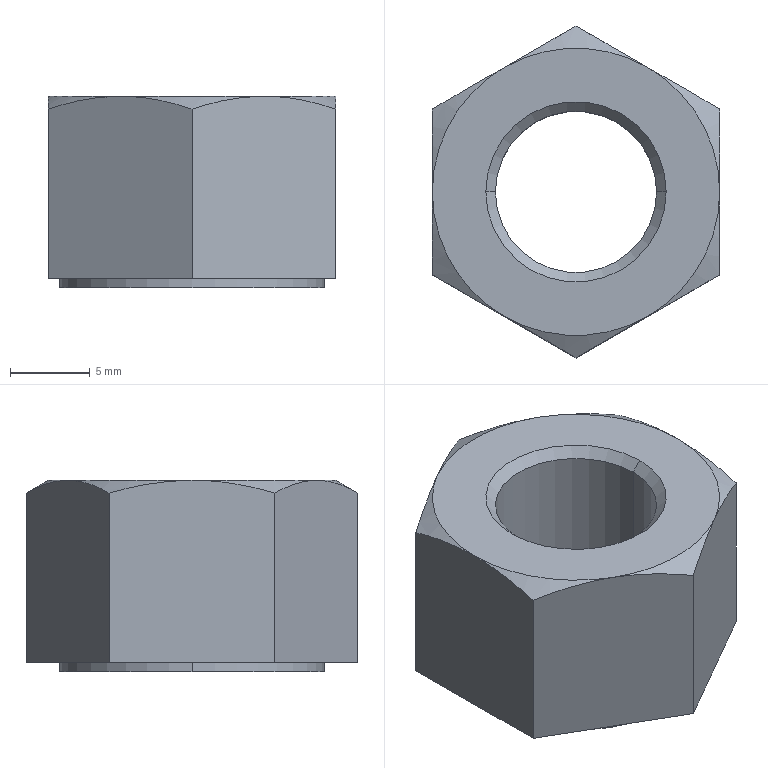Part | SolidWorks | 1 solid | 23 faces | box 18 x 20.785 x 12 mm | volume 2348 mm3 | cone 10 | plane 9 | cylinder 4 | commonest cylinder face diameters 10.106 x2 16.6 x2
STEP:
#1=CARTESIAN_POINT('',(-5.053,0.,11.4));
#2=VERTEX_POINT('',#1);
#3=CARTESIAN_POINT('',(5.053,0.,11.4));
#4=VERTEX_POINT('',#3);
#5=CARTESIAN_POINT('',(0.,0.,11.4));
#6=DIRECTION('',(0.,0.,1.));
#7=DIRECTION('',(-1.,0.,0.));
#8=AXIS2_PLACEMENT_3D('',#5,#6,#7);
#9=CIRCLE('',#8,5.053);
#10=EDGE_CURVE('',#2,#4,#9,.T.);
#11=ORIENTED_EDGE('',*,*,#10,.F.);
#12=CARTESIAN_POINT('',(-5.653,0.,12.));
#13=VERTEX_POINT('',#12);
#14=CARTESIAN_POINT('',(-5.053,0.,11.4));
#15=DIRECTION('',(-0.7071,0.,0.7071));
#16=VECTOR('',#15,1000.);
#17=LINE('',#14,#16);
#18=EDGE_CURVE('',#2,#13,#17,.T.);
#19=ORIENTED_EDGE('',*,*,#18,.T.);
#20=CARTESIAN_POINT('',(5.653,0.,12.));
#21=VERTEX_POINT('',#20);
#22=CARTESIAN_POINT('',(0.,0.,12.));
#23=DIRECTION('',(0.,0.,-1.));
#24=DIRECTION('',(-1.,0.,0.));
#25=AXIS2_PLACEMENT_3D('',#22,#23,#24);
#26=CIRCLE('',#25,5.653);
#27=EDGE_CURVE('',#21,#13,#26,.T.);
#28=ORIENTED_EDGE('',*,*,#27,.F.);
#29=CARTESIAN_POINT('',(5.053,0.,11.4));
#30=DIRECTION('',(0.7071,0.,0.7071));
#31=VECTOR('',#30,1000.);
#32=LINE('',#29,#31);
#33=EDGE_CURVE('',#4,#21,#32,.T.);
#34=ORIENTED_EDGE('',*,*,#33,.F.);
#35=EDGE_LOOP('',(#11,#19,#28,#34));
#36=FACE_OUTER_BOUND('',#35,.T.);
#37=CARTESIAN_POINT('',(0.,0.,11.4));
#38=DIRECTION('',(0.,0.,1.));
#39=DIRECTION('',(1.,0.,0.));
#40=AXIS2_PLACEMENT_3D('',#37,#38,#39);
#41=CONICAL_SURFACE('',#40,5.053,0.7854);
#42=ADVANCED_FACE('',(#36),#41,.F.);
#43=CARTESIAN_POINT('',(5.053,0.,0.6));
#44=VERTEX_POINT('',#43);
#45=CARTESIAN_POINT('',(-5.053,0.,0.6));
#46=VERTEX_POINT('',#45);
#47=CARTESIAN_POINT('',(0.,0.,0.6));
#48=DIRECTION('',(0.,0.,-1.));
#49=DIRECTION('',(-1.,0.,0.));
#50=AXIS2_PLACEMENT_3D('',#47,#48,#49);
#51=CIRCLE('',#50,5.053);
#52=EDGE_CURVE('',#44,#46,#51,.T.);
#53=ORIENTED_EDGE('',*,*,#52,.F.);
#54=CARTESIAN_POINT('',(5.653,0.,0.));
#55=VERTEX_POINT('',#54);
#56=CARTESIAN_POINT('',(5.653,0.,0.));
#57=DIRECTION('',(0.7071,0.,-0.7071));
#58=VECTOR('',#57,1000.);
#59=LINE('',#56,#58);
#60=EDGE_CURVE('',#44,#55,#59,.T.);
#61=ORIENTED_EDGE('',*,*,#60,.T.);
#62=CARTESIAN_POINT('',(-5.653,0.,0.));
#63=VERTEX_POINT('',#62);
#64=CARTESIAN_POINT('',(0.,0.,0.));
#65=DIRECTION('',(0.,0.,1.));
#66=DIRECTION('',(-1.,0.,0.));
#67=AXIS2_PLACEMENT_3D('',#64,#65,#66);
#68=CIRCLE('',#67,5.653);
#69=EDGE_CURVE('',#63,#55,#68,.T.);
#70=ORIENTED_EDGE('',*,*,#69,.F.);
#71=CARTESIAN_POINT('',(-5.653,0.,0.));
#72=DIRECTION('',(-0.7071,0.,-0.7071));
#73=VECTOR('',#72,1000.);
#74=LINE('',#71,#73);
#75=EDGE_CURVE('',#46,#63,#74,.T.);
#76=ORIENTED_EDGE('',*,*,#75,.F.);
#77=EDGE_LOOP('',(#53,#61,#70,#76));
#78=FACE_OUTER_BOUND('',#77,.T.);
#79=CARTESIAN_POINT('',(0.,0.,0.));
#80=DIRECTION('',(0.,0.,-1.));
#81=DIRECTION('',(-1.,0.,0.));
#82=AXIS2_PLACEMENT_3D('',#79,#80,#81);
#83=CONICAL_SURFACE('',#82,5.653,0.7854);
#84=ADVANCED_FACE('',(#78),#83,.F.);
#85=CARTESIAN_POINT('',(8.3,0.,0.6));
#86=VERTEX_POINT('',#85);
#87=CARTESIAN_POINT('',(-8.3,0.,0.6));
#88=VERTEX_POINT('',#87);
#89=CARTESIAN_POINT('',(0.,0.,0.6));
#90=DIRECTION('',(0.,0.,1.));
#91=DIRECTION('',(1.,0.,0.));
#92=AXIS2_PLACEMENT_3D('',#89,#90,#91);
#93=CIRCLE('',#92,8.3);
#94=EDGE_CURVE('',#86,#88,#93,.T.);
#95=ORIENTED_EDGE('',*,*,#94,.F.);
#96=CARTESIAN_POINT('',(8.3,0.,0.));
#97=VERTEX_POINT('',#96);
#98=CARTESIAN_POINT('',(8.3,0.,0.6));
#99=DIRECTION('',(0.,0.,-1.));
#100=VECTOR('',#99,1000.);
#101=LINE('',#98,#100);
#102=EDGE_CURVE('',#86,#97,#101,.T.);
#103=ORIENTED_EDGE('',*,*,#102,.T.);
#104=CARTESIAN_POINT('',(-8.3,0.,0.));
#105=VERTEX_POINT('',#104);
#106=CARTESIAN_POINT('',(0.,0.,0.));
#107=DIRECTION('',(0.,0.,1.));
#108=DIRECTION('',(1.,0.,0.));
#109=AXIS2_PLACEMENT_3D('',#106,#107,#108);
#110=CIRCLE('',#109,8.3);
#111=EDGE_CURVE('',#97,#105,#110,.T.);
#112=ORIENTED_EDGE('',*,*,#111,.T.);
#113=CARTESIAN_POINT('',(-8.3,0.,0.6));
#114=DIRECTION('',(0.,0.,-1.));
#115=VECTOR('',#114,1000.);
#116=LINE('',#113,#115);
#117=EDGE_CURVE('',#88,#105,#116,.T.);
#118=ORIENTED_EDGE('',*,*,#117,.F.);
#119=EDGE_LOOP('',(#95,#103,#112,#118));
#120=FACE_OUTER_BOUND('',#119,.T.);
#121=CARTESIAN_POINT('',(0.,0.,0.6));
#122=DIRECTION('',(0.,0.,-1.));
#123=DIRECTION('',(-1.,0.,0.));
#124=AXIS2_PLACEMENT_3D('',#121,#122,#123);
#125=CYLINDRICAL_SURFACE('',#124,8.3);
#126=ADVANCED_FACE('',(#120),#125,.T.);
#127=ORIENTED_EDGE('',*,*,#10,.T.);
#128=CARTESIAN_POINT('',(5.053,0.,12.));
#129=DIRECTION('',(0.,0.,-1.));
#130=VECTOR('',#129,1000.);
#131=LINE('',#128,#130);
#132=EDGE_CURVE('',#4,#44,#131,.T.);
#133=ORIENTED_EDGE('',*,*,#132,.T.);
#134=ORIENTED_EDGE('',*,*,#52,.T.);
#135=CARTESIAN_POINT('',(-5.053,0.,12.));
#136=DIRECTION('',(0.,0.,-1.));
#137=VECTOR('',#136,1000.);
#138=LINE('',#135,#137);
#139=EDGE_CURVE('',#2,#46,#138,.T.);
#140=ORIENTED_EDGE('',*,*,#139,.F.);
#141=EDGE_LOOP('',(#127,#133,#134,#140));
#142=FACE_OUTER_BOUND('',#141,.T.);
#143=CARTESIAN_POINT('',(0.,0.,12.));
#144=DIRECTION('',(0.,0.,-1.));
#145=DIRECTION('',(-1.,0.,0.));
#146=AXIS2_PLACEMENT_3D('',#143,#144,#145);
#147=CYLINDRICAL_SURFACE('',#146,5.053);
#148=ADVANCED_FACE('',(#142),#147,.F.);
#149=ORIENTED_EDGE('',*,*,#27,.T.);
#150=CARTESIAN_POINT('',(0.,0.,12.));
#151=DIRECTION('',(0.,0.,-1.));
#152=DIRECTION('',(-1.,0.,0.));
#153=AXIS2_PLACEMENT_3D('',#150,#151,#152);
#154=CIRCLE('',#153,5.653);
#155=EDGE_CURVE('',#13,#21,#154,.T.);
#156=ORIENTED_EDGE('',*,*,#155,.T.);
#157=EDGE_LOOP('',(#149,#156));
#158=FACE_BOUND('',#157,.T.);
#159=CARTESIAN_POINT('',(-4.5,7.794,12.));
#160=VERTEX_POINT('',#159);
#161=CARTESIAN_POINT('',(-9.,0.,12.));
#162=VERTEX_POINT('',#161);
#163=CARTESIAN_POINT('',(0.,0.,12.));
#164=DIRECTION('',(0.,0.,1.));
#165=DIRECTION('',(1.,0.,0.));
#166=AXIS2_PLACEMENT_3D('',#163,#164,#165);
#167=CIRCLE('',#166,9.);
#168=EDGE_CURVE('',#160,#162,#167,.T.);
#169=ORIENTED_EDGE('',*,*,#168,.T.);
#170=CARTESIAN_POINT('',(-4.5,-7.794,12.));
#171=VERTEX_POINT('',#170);
#172=CARTESIAN_POINT('',(0.,0.,12.));
#173=DIRECTION('',(0.,0.,1.));
#174=DIRECTION('',(1.,0.,0.));
#175=AXIS2_PLACEMENT_3D('',#172,#173,#174);
#176=CIRCLE('',#175,9.);
#177=EDGE_CURVE('',#162,#171,#176,.T.);
#178=ORIENTED_EDGE('',*,*,#177,.T.);
#179=CARTESIAN_POINT('',(4.5,-7.794,12.));
#180=VERTEX_POINT('',#179);
#181=CARTESIAN_POINT('',(0.,0.,12.));
#182=DIRECTION('',(0.,0.,1.));
#183=DIRECTION('',(1.,0.,0.));
#184=AXIS2_PLACEMENT_3D('',#181,#182,#183);
#185=CIRCLE('',#184,9.);
#186=EDGE_CURVE('',#171,#180,#185,.T.);
#187=ORIENTED_EDGE('',*,*,#186,.T.);
#188=CARTESIAN_POINT('',(9.,0.,12.));
#189=VERTEX_POINT('',#188);
#190=CARTESIAN_POINT('',(0.,0.,12.));
#191=DIRECTION('',(0.,0.,1.));
#192=DIRECTION('',(1.,0.,0.));
#193=AXIS2_PLACEMENT_3D('',#190,#191,#192);
#194=CIRCLE('',#193,9.);
#195=EDGE_CURVE('',#180,#189,#194,.T.);
#196=ORIENTED_EDGE('',*,*,#195,.T.);
#197=CARTESIAN_POINT('',(4.5,7.794,12.));
#198=VERTEX_POINT('',#197);
#199=CARTESIAN_POINT('',(0.,0.,12.));
#200=DIRECTION('',(0.,0.,1.));
#201=DIRECTION('',(1.,0.,0.));
#202=AXIS2_PLACEMENT_3D('',#199,#200,#201);
#203=CIRCLE('',#202,9.);
#204=EDGE_CURVE('',#189,#198,#203,.T.);
#205=ORIENTED_EDGE('',*,*,#204,.T.);
#206=CARTESIAN_POINT('',(0.,0.,12.));
#207=DIRECTION('',(0.,0.,1.));
#208=DIRECTION('',(1.,0.,0.));
#209=AXIS2_PLACEMENT_3D('',#206,#207,#208);
#210=CIRCLE('',#209,9.);
#211=EDGE_CURVE('',#198,#160,#210,.T.);
#212=ORIENTED_EDGE('',*,*,#211,.T.);
#213=EDGE_LOOP('',(#169,#178,#187,#196,#205,#212));
#214=FACE_OUTER_BOUND('',#213,.T.);
#215=CARTESIAN_POINT('',(9.,5.196,12.));
#216=DIRECTION('',(0.,0.,-1.));
#217=DIRECTION('',(-1.,0.,0.));
#218=AXIS2_PLACEMENT_3D('',#215,#216,#217);
#219=PLANE('',#218);
#220=ADVANCED_FACE('',(#158,#214),#219,.F.);
#221=CARTESIAN_POINT('',(9.,5.196,11.196));
#222=VERTEX_POINT('',#221);
#223=CARTESIAN_POINT('',(9.,5.196,11.196));
#224=CARTESIAN_POINT('',(8.264,5.621,11.442));
#225=CARTESIAN_POINT('',(7.522,6.049,11.644));
#226=CARTESIAN_POINT('',(6.024,6.914,11.923));
#227=CARTESIAN_POINT('',(5.267,7.352,12.));
#228=CARTESIAN_POINT('',(4.5,7.794,12.));
#229=B_SPLINE_CURVE_WITH_KNOTS('',3,(#223,#224,#225,#226,#227,#228),.UNSPECIFIED.,.F.,.F.,(4,2,4),(0.000000238,0.002629,0.005258),.UNSPECIFIED.);
#230=EDGE_CURVE('',#222,#198,#229,.T.);
#231=ORIENTED_EDGE('',*,*,#230,.F.);
#232=CARTESIAN_POINT('',(9.,5.196,0.6));
#233=VERTEX_POINT('',#232);
#234=CARTESIAN_POINT('',(9.,5.196,12.));
#235=DIRECTION('',(0.,0.,-1.));
#236=VECTOR('',#235,1000.);
#237=LINE('',#234,#236);
#238=EDGE_CURVE('',#222,#233,#237,.T.);
#239=ORIENTED_EDGE('',*,*,#238,.T.);
#240=CARTESIAN_POINT('',(0.,10.392,0.6));
#241=VERTEX_POINT('',#240);
#242=CARTESIAN_POINT('',(9.,5.196,0.6));
#243=DIRECTION('',(-0.866,0.5,0.));
#244=VECTOR('',#243,1000.);
#245=LINE('',#242,#244);
#246=EDGE_CURVE('',#233,#241,#245,.T.);
#247=ORIENTED_EDGE('',*,*,#246,.T.);
#248=CARTESIAN_POINT('',(0.,10.392,11.196));
#249=VERTEX_POINT('',#248);
#250=CARTESIAN_POINT('',(0.,10.392,12.));
#251=DIRECTION('',(0.,0.,-1.));
#252=VECTOR('',#251,1000.);
#253=LINE('',#250,#252);
#254=EDGE_CURVE('',#249,#241,#253,.T.);
#255=ORIENTED_EDGE('',*,*,#254,.F.);
#256=CARTESIAN_POINT('',(4.5,7.794,12.));
#257=CARTESIAN_POINT('',(4.118,8.015,12.));
#258=CARTESIAN_POINT('',(3.734,8.236,11.981));
#259=CARTESIAN_POINT('',(2.976,8.674,11.907));
#260=CARTESIAN_POINT('',(2.599,8.892,11.853));
#261=CARTESIAN_POINT('',(1.475,9.541,11.643));
#262=CARTESIAN_POINT('',(0.7343,9.968,11.441));
#263=CARTESIAN_POINT('',(0.,10.392,11.196));
#264=B_SPLINE_CURVE_WITH_KNOTS('',3,(#256,#257,#258,#259,#260,#261,#262,#263),.UNSPECIFIED.,.F.,.F.,(4,2,2,4),(0.005258,0.006567,0.007877,0.0105),.UNSPECIFIED.);
#265=EDGE_CURVE('',#198,#249,#264,.T.);
#266=ORIENTED_EDGE('',*,*,#265,.F.);
#267=EDGE_LOOP('',(#231,#239,#247,#255,#266));
#268=FACE_OUTER_BOUND('',#267,.T.);
#269=CARTESIAN_POINT('',(9.,5.196,12.));
#270=DIRECTION('',(-0.5,-0.866,0.));
#271=DIRECTION('',(0.866,-0.5,0.));
#272=AXIS2_PLACEMENT_3D('',#269,#270,#271);
#273=PLANE('',#272);
#274=ADVANCED_FACE('',(#268),#273,.F.);
#275=CARTESIAN_POINT('',(0.,10.392,11.196));
#276=CARTESIAN_POINT('',(-0.7361,9.967,11.442));
#277=CARTESIAN_POINT('',(-1.478,9.539,11.644));
#278=CARTESIAN_POINT('',(-2.976,8.674,11.923));
#279=CARTESIAN_POINT('',(-3.733,8.237,12.));
#280=CARTESIAN_POINT('',(-4.5,7.794,12.));
#281=B_SPLINE_CURVE_WITH_KNOTS('',3,(#275,#276,#277,#278,#279,#280),.UNSPECIFIED.,.F.,.F.,(4,2,4),(0.000000238,0.002629,0.005258),.UNSPECIFIED.);
#282=EDGE_CURVE('',#249,#160,#281,.T.);
#283=ORIENTED_EDGE('',*,*,#282,.F.);
#284=ORIENTED_EDGE('',*,*,#254,.T.);
#285=CARTESIAN_POINT('',(-9.,5.196,0.6));
#286=VERTEX_POINT('',#285);
#287=CARTESIAN_POINT('',(0.,10.392,0.6));
#288=DIRECTION('',(-0.866,-0.5,0.));
#289=VECTOR('',#288,1000.);
#290=LINE('',#287,#289);
#291=EDGE_CURVE('',#241,#286,#290,.T.);
#292=ORIENTED_EDGE('',*,*,#291,.T.);
#293=CARTESIAN_POINT('',(-9.,5.196,11.196));
#294=VERTEX_POINT('',#293);
#295=CARTESIAN_POINT('',(-9.,5.196,12.));
#296=DIRECTION('',(0.,0.,-1.));
#297=VECTOR('',#296,1000.);
#298=LINE('',#295,#297);
#299=EDGE_CURVE('',#294,#286,#298,.T.);
#300=ORIENTED_EDGE('',*,*,#299,.F.);
#301=CARTESIAN_POINT('',(-4.5,7.794,12.));
#302=CARTESIAN_POINT('',(-4.882,7.574,12.));
#303=CARTESIAN_POINT('',(-5.266,7.352,11.981));
#304=CARTESIAN_POINT('',(-6.024,6.914,11.907));
#305=CARTESIAN_POINT('',(-6.401,6.697,11.853));
#306=CARTESIAN_POINT('',(-7.525,6.048,11.643));
#307=CARTESIAN_POINT('',(-8.266,5.62,11.441));
#308=CARTESIAN_POINT('',(-9.,5.196,11.196));
#309=B_SPLINE_CURVE_WITH_KNOTS('',3,(#301,#302,#303,#304,#305,#306,#307,#308),.UNSPECIFIED.,.F.,.F.,(4,2,2,4),(0.005258,0.006567,0.007877,0.0105),.UNSPECIFIED.);
#310=EDGE_CURVE('',#160,#294,#309,.T.);
#311=ORIENTED_EDGE('',*,*,#310,.F.);
#312=EDGE_LOOP('',(#283,#284,#292,#300,#311));
#313=FACE_OUTER_BOUND('',#312,.T.);
#314=CARTESIAN_POINT('',(0.,10.392,12.));
#315=DIRECTION('',(0.5,-0.866,0.));
#316=DIRECTION('',(0.866,0.5,0.));
#317=AXIS2_PLACEMENT_3D('',#314,#315,#316);
#318=PLANE('',#317);
#319=ADVANCED_FACE('',(#313),#318,.F.);
#320=CARTESIAN_POINT('',(-9.,5.196,11.196));
#321=CARTESIAN_POINT('',(-9.,4.356,11.439));
#322=CARTESIAN_POINT('',(-9.,3.505,11.641));
#323=CARTESIAN_POINT('',(-9.,2.204,11.852));
#324=CARTESIAN_POINT('',(-9.,1.766,11.907));
#325=CARTESIAN_POINT('',(-9.,0.8817,11.981));
#326=CARTESIAN_POINT('',(-9.,0.4398,12.));
#327=CARTESIAN_POINT('',(-9.,0.,12.));
#328=B_SPLINE_CURVE_WITH_KNOTS('',3,(#320,#321,#322,#323,#324,#325,#326,#327),.UNSPECIFIED.,.F.,.F.,(4,2,2,4),(0.03023,0.03286,0.03418,0.03549),.UNSPECIFIED.);
#329=EDGE_CURVE('',#294,#162,#328,.T.);
#330=ORIENTED_EDGE('',*,*,#329,.F.);
#331=ORIENTED_EDGE('',*,*,#299,.T.);
#332=CARTESIAN_POINT('',(-9.,-5.196,0.6));
#333=VERTEX_POINT('',#332);
#334=CARTESIAN_POINT('',(-9.,5.196,0.6));
#335=DIRECTION('',(0.,-1.,0.));
#336=VECTOR('',#335,1000.);
#337=LINE('',#334,#336);
#338=EDGE_CURVE('',#286,#333,#337,.T.);
#339=ORIENTED_EDGE('',*,*,#338,.T.);
#340=CARTESIAN_POINT('',(-9.,-5.196,11.196));
#341=VERTEX_POINT('',#340);
#342=CARTESIAN_POINT('',(-9.,-5.196,12.));
#343=DIRECTION('',(0.,0.,-1.));
#344=VECTOR('',#343,1000.);
#345=LINE('',#342,#344);
#346=EDGE_CURVE('',#341,#333,#345,.T.);
#347=ORIENTED_EDGE('',*,*,#346,.F.);
#348=CARTESIAN_POINT('',(-9.,0.,12.));
#349=CARTESIAN_POINT('',(-9.,-0.8789,12.));
#350=CARTESIAN_POINT('',(-9.,-1.751,11.924));
#351=CARTESIAN_POINT('',(-9.,-3.485,11.645));
#352=CARTESIAN_POINT('',(-9.,-4.35,11.44));
#353=CARTESIAN_POINT('',(-9.,-5.196,11.196));
#354=B_SPLINE_CURVE_WITH_KNOTS('',3,(#348,#349,#350,#351,#352,#353),.UNSPECIFIED.,.F.,.F.,(4,2,4),(0.03549,0.03812,0.04075),.UNSPECIFIED.);
#355=EDGE_CURVE('',#162,#341,#354,.T.);
#356=ORIENTED_EDGE('',*,*,#355,.F.);
#357=EDGE_LOOP('',(#330,#331,#339,#347,#356));
#358=FACE_OUTER_BOUND('',#357,.T.);
#359=CARTESIAN_POINT('',(-9.,5.196,12.));
#360=DIRECTION('',(1.,0.,0.));
#361=DIRECTION('',(0.,0.,-1.));
#362=AXIS2_PLACEMENT_3D('',#359,#360,#361);
#363=PLANE('',#362);
#364=ADVANCED_FACE('',(#358),#363,.F.);
#365=CARTESIAN_POINT('',(-9.,-5.196,11.196));
#366=CARTESIAN_POINT('',(-8.264,-5.621,11.442));
#367=CARTESIAN_POINT('',(-7.522,-6.049,11.644));
#368=CARTESIAN_POINT('',(-6.024,-6.914,11.923));
#369=CARTESIAN_POINT('',(-5.267,-7.352,12.));
#370=CARTESIAN_POINT('',(-4.5,-7.794,12.));
#371=B_SPLINE_CURVE_WITH_KNOTS('',3,(#365,#366,#367,#368,#369,#370),.UNSPECIFIED.,.F.,.F.,(4,2,4),(0.000000238,0.002629,0.005258),.UNSPECIFIED.);
#372=EDGE_CURVE('',#341,#171,#371,.T.);
#373=ORIENTED_EDGE('',*,*,#372,.F.);
#374=ORIENTED_EDGE('',*,*,#346,.T.);
#375=CARTESIAN_POINT('',(0.,-10.392,0.6));
#376=VERTEX_POINT('',#375);
#377=CARTESIAN_POINT('',(-9.,-5.196,0.6));
#378=DIRECTION('',(0.866,-0.5,0.));
#379=VECTOR('',#378,1000.);
#380=LINE('',#377,#379);
#381=EDGE_CURVE('',#333,#376,#380,.T.);
#382=ORIENTED_EDGE('',*,*,#381,.T.);
#383=CARTESIAN_POINT('',(0.,-10.392,11.196));
#384=VERTEX_POINT('',#383);
#385=CARTESIAN_POINT('',(0.,-10.392,12.));
#386=DIRECTION('',(0.,0.,-1.));
#387=VECTOR('',#386,1000.);
#388=LINE('',#385,#387);
#389=EDGE_CURVE('',#384,#376,#388,.T.);
#390=ORIENTED_EDGE('',*,*,#389,.F.);
#391=CARTESIAN_POINT('',(-4.5,-7.794,12.));
#392=CARTESIAN_POINT('',(-4.118,-8.015,12.));
#393=CARTESIAN_POINT('',(-3.734,-8.236,11.981));
#394=CARTESIAN_POINT('',(-2.976,-8.674,11.907));
#395=CARTESIAN_POINT('',(-2.599,-8.892,11.853));
#396=CARTESIAN_POINT('',(-1.475,-9.541,11.643));
#397=CARTESIAN_POINT('',(-0.7343,-9.968,11.441));
#398=CARTESIAN_POINT('',(0.,-10.392,11.196));
#399=B_SPLINE_CURVE_WITH_KNOTS('',3,(#391,#392,#393,#394,#395,#396,#397,#398),.UNSPECIFIED.,.F.,.F.,(4,2,2,4),(0.005258,0.006567,0.007877,0.0105),.UNSPECIFIED.);
#400=EDGE_CURVE('',#171,#384,#399,.T.);
#401=ORIENTED_EDGE('',*,*,#400,.F.);
#402=EDGE_LOOP('',(#373,#374,#382,#390,#401));
#403=FACE_OUTER_BOUND('',#402,.T.);
#404=CARTESIAN_POINT('',(-9.,-5.196,12.));
#405=DIRECTION('',(0.5,0.866,0.));
#406=DIRECTION('',(-0.866,0.5,0.));
#407=AXIS2_PLACEMENT_3D('',#404,#405,#406);
#408=PLANE('',#407);
#409=ADVANCED_FACE('',(#403),#408,.F.);
#410=CARTESIAN_POINT('',(0.,-10.392,11.196));
#411=CARTESIAN_POINT('',(0.7361,-9.967,11.442));
#412=CARTESIAN_POINT('',(1.478,-9.539,11.644));
#413=CARTESIAN_POINT('',(2.976,-8.674,11.923));
#414=CARTESIAN_POINT('',(3.733,-8.237,12.));
#415=CARTESIAN_POINT('',(4.5,-7.794,12.));
#416=B_SPLINE_CURVE_WITH_KNOTS('',3,(#410,#411,#412,#413,#414,#415),.UNSPECIFIED.,.F.,.F.,(4,2,4),(0.000000238,0.002629,0.005258),.UNSPECIFIED.);
#417=EDGE_CURVE('',#384,#180,#416,.T.);
#418=ORIENTED_EDGE('',*,*,#417,.F.);
#419=ORIENTED_EDGE('',*,*,#389,.T.);
#420=CARTESIAN_POINT('',(9.,-5.196,0.6));
#421=VERTEX_POINT('',#420);
#422=CARTESIAN_POINT('',(0.,-10.392,0.6));
#423=DIRECTION('',(0.866,0.5,0.));
#424=VECTOR('',#423,1000.);
#425=LINE('',#422,#424);
#426=EDGE_CURVE('',#376,#421,#425,.T.);
#427=ORIENTED_EDGE('',*,*,#426,.T.);
#428=CARTESIAN_POINT('',(9.,-5.196,11.196));
#429=VERTEX_POINT('',#428);
#430=CARTESIAN_POINT('',(9.,-5.196,12.));
#431=DIRECTION('',(0.,0.,-1.));
#432=VECTOR('',#431,1000.);
#433=LINE('',#430,#432);
#434=EDGE_CURVE('',#429,#421,#433,.T.);
#435=ORIENTED_EDGE('',*,*,#434,.F.);
#436=CARTESIAN_POINT('',(4.5,-7.794,12.));
#437=CARTESIAN_POINT('',(4.882,-7.574,12.));
#438=CARTESIAN_POINT('',(5.266,-7.352,11.981));
#439=CARTESIAN_POINT('',(6.024,-6.914,11.907));
#440=CARTESIAN_POINT('',(6.401,-6.697,11.853));
#441=CARTESIAN_POINT('',(7.525,-6.048,11.643));
#442=CARTESIAN_POINT('',(8.266,-5.62,11.441));
#443=CARTESIAN_POINT('',(9.,-5.196,11.196));
#444=B_SPLINE_CURVE_WITH_KNOTS('',3,(#436,#437,#438,#439,#440,#441,#442,#443),.UNSPECIFIED.,.F.,.F.,(4,2,2,4),(0.005258,0.006567,0.007877,0.0105),.UNSPECIFIED.);
#445=EDGE_CURVE('',#180,#429,#444,.T.);
#446=ORIENTED_EDGE('',*,*,#445,.F.);
#447=EDGE_LOOP('',(#418,#419,#427,#435,#446));
#448=FACE_OUTER_BOUND('',#447,.T.);
#449=CARTESIAN_POINT('',(0.,-10.392,12.));
#450=DIRECTION('',(-0.5,0.866,0.));
#451=DIRECTION('',(-0.866,-0.5,0.));
#452=AXIS2_PLACEMENT_3D('',#449,#450,#451);
#453=PLANE('',#452);
#454=ADVANCED_FACE('',(#448),#453,.F.);
#455=CARTESIAN_POINT('',(9.,-5.196,11.196));
#456=CARTESIAN_POINT('',(9.,-4.35,11.44));
#457=CARTESIAN_POINT('',(9.,-3.485,11.645));
#458=CARTESIAN_POINT('',(9.,-1.751,11.924));
#459=CARTESIAN_POINT('',(9.,-0.8789,12.));
#460=CARTESIAN_POINT('',(9.,0.,12.));
#461=B_SPLINE_CURVE_WITH_KNOTS('',3,(#455,#456,#457,#458,#459,#460),.UNSPECIFIED.,.F.,.F.,(4,2,4),(0.009551,0.01218,0.01481),.UNSPECIFIED.);
#462=EDGE_CURVE('',#429,#189,#461,.T.);
#463=ORIENTED_EDGE('',*,*,#462,.F.);
#464=ORIENTED_EDGE('',*,*,#434,.T.);
#465=CARTESIAN_POINT('',(9.,-5.196,0.6));
#466=DIRECTION('',(0.,1.,0.));
#467=VECTOR('',#466,1000.);
#468=LINE('',#465,#467);
#469=EDGE_CURVE('',#421,#233,#468,.T.);
#470=ORIENTED_EDGE('',*,*,#469,.T.);
#471=ORIENTED_EDGE('',*,*,#238,.F.);
#472=CARTESIAN_POINT('',(9.,0.,12.));
#473=CARTESIAN_POINT('',(9.,0.4398,12.));
#474=CARTESIAN_POINT('',(9.,0.8817,11.981));
#475=CARTESIAN_POINT('',(9.,1.766,11.907));
#476=CARTESIAN_POINT('',(9.,2.204,11.852));
#477=CARTESIAN_POINT('',(9.,3.505,11.641));
#478=CARTESIAN_POINT('',(9.,4.356,11.439));
#479=CARTESIAN_POINT('',(9.,5.196,11.196));
#480=B_SPLINE_CURVE_WITH_KNOTS('',3,(#472,#473,#474,#475,#476,#477,#478,#479),.UNSPECIFIED.,.F.,.F.,(4,2,2,4),(0.01481,0.01613,0.01744,0.02007),.UNSPECIFIED.);
#481=EDGE_CURVE('',#189,#222,#480,.T.);
#482=ORIENTED_EDGE('',*,*,#481,.F.);
#483=EDGE_LOOP('',(#463,#464,#470,#471,#482));
#484=FACE_OUTER_BOUND('',#483,.T.);
#485=CARTESIAN_POINT('',(9.,-5.196,12.));
#486=DIRECTION('',(-1.,0.,0.));
#487=DIRECTION('',(0.,-1.,0.));
#488=AXIS2_PLACEMENT_3D('',#485,#486,#487);
#489=PLANE('',#488);
#490=ADVANCED_FACE('',(#484),#489,.F.);
#491=ORIENTED_EDGE('',*,*,#69,.T.);
#492=CARTESIAN_POINT('',(0.,0.,0.));
#493=DIRECTION('',(0.,0.,1.));
#494=DIRECTION('',(-1.,0.,0.));
#495=AXIS2_PLACEMENT_3D('',#492,#493,#494);
#496=CIRCLE('',#495,5.653);
#497=EDGE_CURVE('',#55,#63,#496,.T.);
#498=ORIENTED_EDGE('',*,*,#497,.T.);
#499=EDGE_LOOP('',(#491,#498));
#500=FACE_BOUND('',#499,.T.);
#501=CARTESIAN_POINT('',(0.,0.,0.));
#502=DIRECTION('',(0.,0.,1.));
#503=DIRECTION('',(1.,0.,0.));
#504=AXIS2_PLACEMENT_3D('',#501,#502,#503);
#505=CIRCLE('',#504,8.3);
#506=EDGE_CURVE('',#105,#97,#505,.T.);
#507=ORIENTED_EDGE('',*,*,#506,.F.);
#508=ORIENTED_EDGE('',*,*,#111,.F.);
#509=EDGE_LOOP('',(#507,#508));
#510=FACE_OUTER_BOUND('',#509,.T.);
#511=CARTESIAN_POINT('',(9.,5.196,0.));
#512=DIRECTION('',(0.,0.,-1.));
#513=DIRECTION('',(-1.,0.,0.));
#514=AXIS2_PLACEMENT_3D('',#511,#512,#513);
#515=PLANE('',#514);
#516=ADVANCED_FACE('',(#500,#510),#515,.T.);
#517=ORIENTED_EDGE('',*,*,#132,.F.);
#518=CARTESIAN_POINT('',(0.,0.,11.4));
#519=DIRECTION('',(0.,0.,1.));
#520=DIRECTION('',(-1.,0.,0.));
#521=AXIS2_PLACEMENT_3D('',#518,#519,#520);
#522=CIRCLE('',#521,5.053);
#523=EDGE_CURVE('',#4,#2,#522,.T.);
#524=ORIENTED_EDGE('',*,*,#523,.T.);
#525=ORIENTED_EDGE('',*,*,#139,.T.);
#526=CARTESIAN_POINT('',(0.,0.,0.6));
#527=DIRECTION('',(0.,0.,-1.));
#528=DIRECTION('',(-1.,0.,0.));
#529=AXIS2_PLACEMENT_3D('',#526,#527,#528);
#530=CIRCLE('',#529,5.053);
#531=EDGE_CURVE('',#46,#44,#530,.T.);
#532=ORIENTED_EDGE('',*,*,#531,.T.);
#533=EDGE_LOOP('',(#517,#524,#525,#532));
#534=FACE_OUTER_BOUND('',#533,.T.);
#535=CARTESIAN_POINT('',(0.,0.,12.));
#536=DIRECTION('',(0.,0.,-1.));
#537=DIRECTION('',(-1.,0.,0.));
#538=AXIS2_PLACEMENT_3D('',#535,#536,#537);
#539=CYLINDRICAL_SURFACE('',#538,5.053);
#540=ADVANCED_FACE('',(#534),#539,.F.);
#541=CARTESIAN_POINT('',(0.,0.,0.6));
#542=DIRECTION('',(0.,0.,1.));
#543=DIRECTION('',(1.,0.,0.));
#544=AXIS2_PLACEMENT_3D('',#541,#542,#543);
#545=CIRCLE('',#544,8.3);
#546=EDGE_CURVE('',#88,#86,#545,.T.);
#547=ORIENTED_EDGE('',*,*,#546,.T.);
#548=ORIENTED_EDGE('',*,*,#94,.T.);
#549=EDGE_LOOP('',(#547,#548));
#550=FACE_BOUND('',#549,.T.);
#551=ORIENTED_EDGE('',*,*,#469,.F.);
#552=ORIENTED_EDGE('',*,*,#426,.F.);
#553=ORIENTED_EDGE('',*,*,#381,.F.);
#554=ORIENTED_EDGE('',*,*,#338,.F.);
#555=ORIENTED_EDGE('',*,*,#291,.F.);
#556=ORIENTED_EDGE('',*,*,#246,.F.);
#557=EDGE_LOOP('',(#551,#552,#553,#554,#555,#556));
#558=FACE_OUTER_BOUND('',#557,.T.);
#559=CARTESIAN_POINT('',(0.,0.,0.6));
#560=DIRECTION('',(0.,0.,1.));
#561=DIRECTION('',(1.,0.,0.));
#562=AXIS2_PLACEMENT_3D('',#559,#560,#561);
#563=PLANE('',#562);
#564=ADVANCED_FACE('',(#550,#558),#563,.F.);
#565=ORIENTED_EDGE('',*,*,#102,.F.);
#566=ORIENTED_EDGE('',*,*,#546,.F.);
#567=ORIENTED_EDGE('',*,*,#117,.T.);
#568=ORIENTED_EDGE('',*,*,#506,.T.);
#569=EDGE_LOOP('',(#565,#566,#567,#568));
#570=FACE_OUTER_BOUND('',#569,.T.);
#571=CARTESIAN_POINT('',(0.,0.,0.6));
#572=DIRECTION('',(0.,0.,-1.));
#573=DIRECTION('',(-1.,0.,0.));
#574=AXIS2_PLACEMENT_3D('',#571,#572,#573);
#575=CYLINDRICAL_SURFACE('',#574,8.3);
#576=ADVANCED_FACE('',(#570),#575,.T.);
#577=ORIENTED_EDGE('',*,*,#230,.T.);
#578=ORIENTED_EDGE('',*,*,#204,.F.);
#579=ORIENTED_EDGE('',*,*,#481,.T.);
#580=EDGE_LOOP('',(#577,#578,#579));
#581=FACE_OUTER_BOUND('',#580,.T.);
#582=CARTESIAN_POINT('',(0.,0.,12.));
#583=DIRECTION('',(0.,0.,-1.));
#584=DIRECTION('',(1.,0.,0.));
#585=AXIS2_PLACEMENT_3D('',#582,#583,#584);
#586=CONICAL_SURFACE('',#585,9.,1.047);
#587=ADVANCED_FACE('',(#581),#586,.T.);
#588=ORIENTED_EDGE('',*,*,#445,.T.);
#589=ORIENTED_EDGE('',*,*,#462,.T.);
#590=ORIENTED_EDGE('',*,*,#195,.F.);
#591=EDGE_LOOP('',(#588,#589,#590));
#592=FACE_OUTER_BOUND('',#591,.T.);
#593=CARTESIAN_POINT('',(0.,0.,12.));
#594=DIRECTION('',(0.,0.,-1.));
#595=DIRECTION('',(1.,0.,0.));
#596=AXIS2_PLACEMENT_3D('',#593,#594,#595);
#597=CONICAL_SURFACE('',#596,9.,1.047);
#598=ADVANCED_FACE('',(#592),#597,.T.);
#599=ORIENTED_EDGE('',*,*,#400,.T.);
#600=ORIENTED_EDGE('',*,*,#417,.T.);
#601=ORIENTED_EDGE('',*,*,#186,.F.);
#602=EDGE_LOOP('',(#599,#600,#601));
#603=FACE_OUTER_BOUND('',#602,.T.);
#604=CARTESIAN_POINT('',(0.,0.,12.));
#605=DIRECTION('',(0.,0.,-1.));
#606=DIRECTION('',(1.,0.,0.));
#607=AXIS2_PLACEMENT_3D('',#604,#605,#606);
#608=CONICAL_SURFACE('',#607,9.,1.047);
#609=ADVANCED_FACE('',(#603),#608,.T.);
#610=ORIENTED_EDGE('',*,*,#355,.T.);
#611=ORIENTED_EDGE('',*,*,#372,.T.);
#612=ORIENTED_EDGE('',*,*,#177,.F.);
#613=EDGE_LOOP('',(#610,#611,#612));
#614=FACE_OUTER_BOUND('',#613,.T.);
#615=CARTESIAN_POINT('',(0.,0.,12.));
#616=DIRECTION('',(0.,0.,-1.));
#617=DIRECTION('',(1.,0.,0.));
#618=AXIS2_PLACEMENT_3D('',#615,#616,#617);
#619=CONICAL_SURFACE('',#618,9.,1.047);
#620=ADVANCED_FACE('',(#614),#619,.T.);
#621=ORIENTED_EDGE('',*,*,#310,.T.);
#622=ORIENTED_EDGE('',*,*,#329,.T.);
#623=ORIENTED_EDGE('',*,*,#168,.F.);
#624=EDGE_LOOP('',(#621,#622,#623));
#625=FACE_OUTER_BOUND('',#624,.T.);
#626=CARTESIAN_POINT('',(0.,0.,12.));
#627=DIRECTION('',(0.,0.,-1.));
#628=DIRECTION('',(1.,0.,0.));
#629=AXIS2_PLACEMENT_3D('',#626,#627,#628);
#630=CONICAL_SURFACE('',#629,9.,1.047);
#631=ADVANCED_FACE('',(#625),#630,.T.);
#632=ORIENTED_EDGE('',*,*,#265,.T.);
#633=ORIENTED_EDGE('',*,*,#282,.T.);
#634=ORIENTED_EDGE('',*,*,#211,.F.);
#635=EDGE_LOOP('',(#632,#633,#634));
#636=FACE_OUTER_BOUND('',#635,.T.);
#637=CARTESIAN_POINT('',(0.,0.,12.));
#638=DIRECTION('',(0.,0.,-1.));
#639=DIRECTION('',(1.,0.,0.));
#640=AXIS2_PLACEMENT_3D('',#637,#638,#639);
#641=CONICAL_SURFACE('',#640,9.,1.047);
#642=ADVANCED_FACE('',(#636),#641,.T.);
#643=ORIENTED_EDGE('',*,*,#60,.F.);
#644=ORIENTED_EDGE('',*,*,#531,.F.);
#645=ORIENTED_EDGE('',*,*,#75,.T.);
#646=ORIENTED_EDGE('',*,*,#497,.F.);
#647=EDGE_LOOP('',(#643,#644,#645,#646));
#648=FACE_OUTER_BOUND('',#647,.T.);
#649=CARTESIAN_POINT('',(0.,0.,0.));
#650=DIRECTION('',(0.,0.,-1.));
#651=DIRECTION('',(-1.,0.,0.));
#652=AXIS2_PLACEMENT_3D('',#649,#650,#651);
#653=CONICAL_SURFACE('',#652,5.653,0.7854);
#654=ADVANCED_FACE('',(#648),#653,.F.);
#655=ORIENTED_EDGE('',*,*,#18,.F.);
#656=ORIENTED_EDGE('',*,*,#523,.F.);
#657=ORIENTED_EDGE('',*,*,#33,.T.);
#658=ORIENTED_EDGE('',*,*,#155,.F.);
#659=EDGE_LOOP('',(#655,#656,#657,#658));
#660=FACE_OUTER_BOUND('',#659,.T.);
#661=CARTESIAN_POINT('',(0.,0.,11.4));
#662=DIRECTION('',(0.,0.,1.));
#663=DIRECTION('',(1.,0.,0.));
#664=AXIS2_PLACEMENT_3D('',#661,#662,#663);
#665=CONICAL_SURFACE('',#664,5.053,0.7854);
#666=ADVANCED_FACE('',(#660),#665,.F.);
#667=CLOSED_SHELL('',(#42,#84,#126,#148,#220,#274,#319,#364,#409,#454,#490,#516,#540,#564,#576,#587,#598,#609,#620,#631,#642,#654,#666));
#668=MANIFOLD_SOLID_BREP('',#667);
#669=CARTESIAN_POINT('',(0.,0.,0.));
#670=DIRECTION('',(0.,0.,1.));
#671=DIRECTION('',(1.,0.,0.));
#672=AXIS2_PLACEMENT_3D('',#669,#670,#671);
#673=(LENGTH_UNIT()NAMED_UNIT(*)SI_UNIT(.MILLI.,.METRE.));
#674=UNCERTAINTY_MEASURE_WITH_UNIT(LENGTH_MEASURE(0.00001),#673,'','');
#675=(NAMED_UNIT(*)PLANE_ANGLE_UNIT()SI_UNIT($,.RADIAN.));
#676=(NAMED_UNIT(*)SI_UNIT($,.STERADIAN.)SOLID_ANGLE_UNIT());
#677=(GEOMETRIC_REPRESENTATION_CONTEXT(3)GLOBAL_UNCERTAINTY_ASSIGNED_CONTEXT((#674))GLOBAL_UNIT_ASSIGNED_CONTEXT((#673,#675,#676))REPRESENTATION_CONTEXT('',''));
#678=ADVANCED_BREP_SHAPE_REPRESENTATION('',(#668,#672),#677);